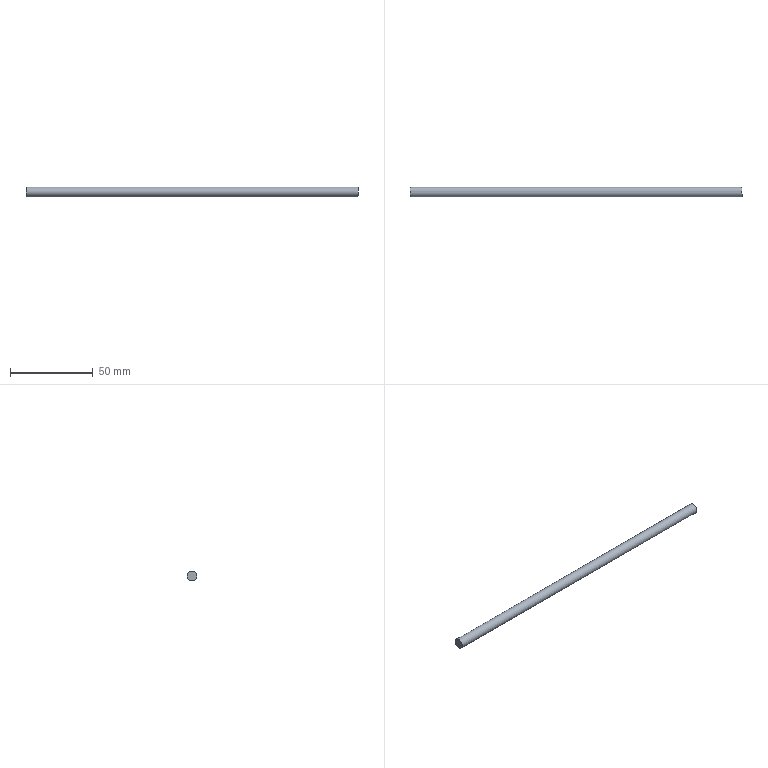Part | NX | features solid 2 | 1 solid | 3 faces | box 200 x 6 x 6 mm | volume 5655 mm3 | plane 2 | cylinder 1 | commonest cylinder face diameters 6 x1
STEP:
#1=CARTESIAN_POINT('',(85.,98.,-100.));
#2=VERTEX_POINT('',#1);
#3=CARTESIAN_POINT('',(85.,95.,-100.));
#4=DIRECTION('',(1.,0.,0.));
#5=DIRECTION('',(0.,1.,0.));
#6=AXIS2_PLACEMENT_3D('',#3,#4,#5);
#7=CIRCLE('',#6,3.);
#8=EDGE_CURVE('',#2,#2,#7,.T.);
#9=ORIENTED_EDGE('',*,*,#8,.F.);
#10=EDGE_LOOP('',(#9));
#11=FACE_BOUND('',#10,.T.);
#12=CARTESIAN_POINT('',(-115.,98.,-100.));
#13=VERTEX_POINT('',#12);
#14=CARTESIAN_POINT('',(-115.,95.,-100.));
#15=DIRECTION('',(1.,0.,0.));
#16=DIRECTION('',(0.,1.,0.));
#17=AXIS2_PLACEMENT_3D('',#14,#15,#16);
#18=CIRCLE('',#17,3.);
#19=EDGE_CURVE('',#13,#13,#18,.T.);
#20=ORIENTED_EDGE('',*,*,#19,.T.);
#21=EDGE_LOOP('',(#20));
#22=FACE_BOUND('',#21,.T.);
#23=CARTESIAN_POINT('',(85.,95.,-100.));
#24=DIRECTION('',(-1.,0.,0.));
#25=DIRECTION('',(0.,-1.,0.));
#26=AXIS2_PLACEMENT_3D('',#23,#24,#25);
#27=CYLINDRICAL_SURFACE('',#26,3.);
#28=ADVANCED_FACE('',(#11,#22),#27,.T.);
#29=ORIENTED_EDGE('',*,*,#8,.T.);
#30=EDGE_LOOP('',(#29));
#31=FACE_BOUND('',#30,.T.);
#32=CARTESIAN_POINT('',(85.,95.,-100.));
#33=DIRECTION('',(1.,0.,0.));
#34=DIRECTION('',(0.,1.,0.));
#35=AXIS2_PLACEMENT_3D('',#32,#33,#34);
#36=PLANE('',#35);
#37=ADVANCED_FACE('',(#31),#36,.T.);
#38=ORIENTED_EDGE('',*,*,#19,.F.);
#39=EDGE_LOOP('',(#38));
#40=FACE_BOUND('',#39,.T.);
#41=CARTESIAN_POINT('',(-115.,95.,-100.));
#42=DIRECTION('',(1.,0.,0.));
#43=DIRECTION('',(0.,1.,0.));
#44=AXIS2_PLACEMENT_3D('',#41,#42,#43);
#45=PLANE('',#44);
#46=ADVANCED_FACE('',(#40),#45,.F.);
#47=CLOSED_SHELL('',(#28,#37,#46));
#48=MANIFOLD_SOLID_BREP('',#47);
#49=(LENGTH_UNIT()NAMED_UNIT(*)SI_UNIT(.MILLI.,.METRE.));
#50=UNCERTAINTY_MEASURE_WITH_UNIT(LENGTH_MEASURE(0.00001),#49,'','');
#51=(NAMED_UNIT(*)PLANE_ANGLE_UNIT()SI_UNIT($,.RADIAN.));
#52=(NAMED_UNIT(*)SI_UNIT($,.STERADIAN.)SOLID_ANGLE_UNIT());
#53=(GEOMETRIC_REPRESENTATION_CONTEXT(3)GLOBAL_UNCERTAINTY_ASSIGNED_CONTEXT((#50))GLOBAL_UNIT_ASSIGNED_CONTEXT((#49,#51,#52))REPRESENTATION_CONTEXT('',''));
#54=ADVANCED_BREP_SHAPE_REPRESENTATION('',(#48),#53);